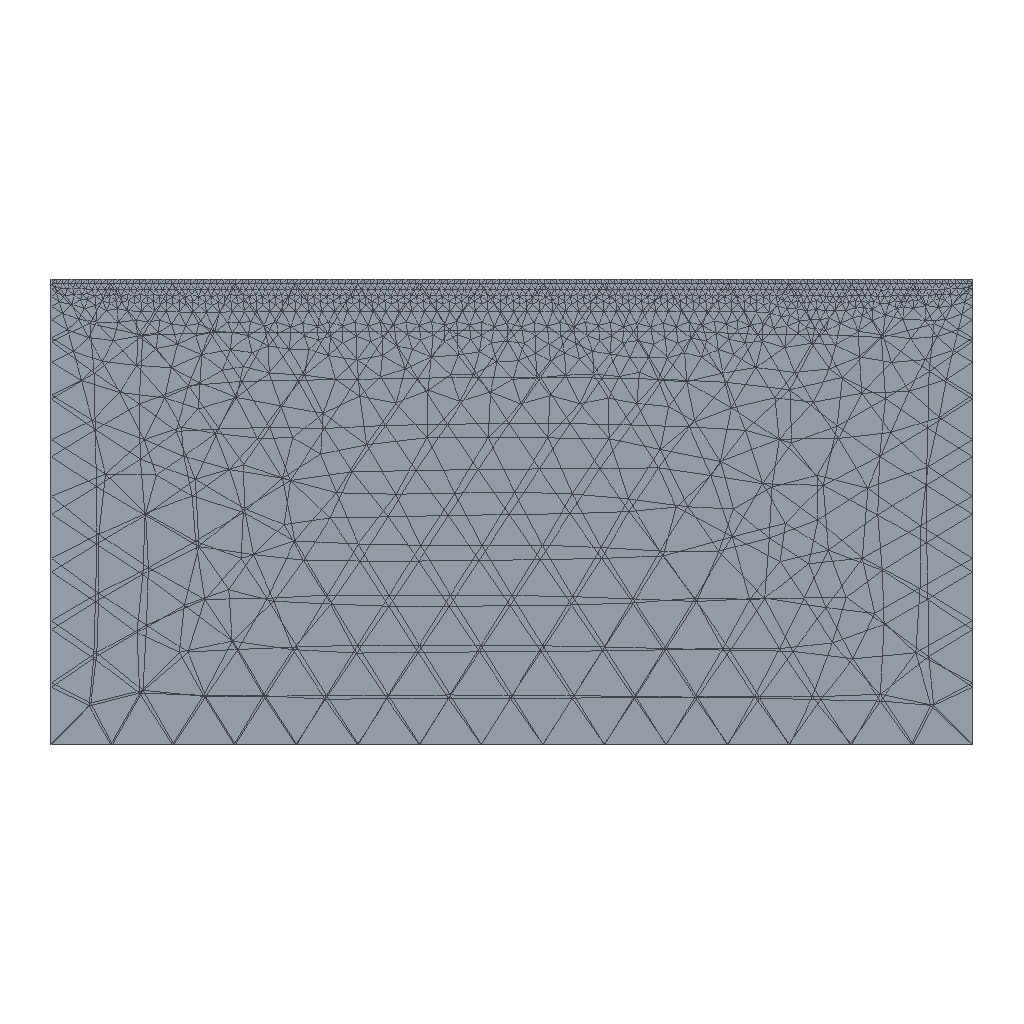Simulation study | comsol
Set-up summary:
category,name,step,type,value,unit,region
solver,comsol,,COMSOL Multiphysics 6.4 (Build: 293)
units,SI; geometry length unit m,,stated,COMSOL default unit system (SI)
analysis,Study 1,,Transient,space_dimension=2D
load_step,std1/time,std1/time,Transient,"type=Transient; times=range(0,5,60)"
analysis,Study 2,,Transient,space_dimension=2D
load_step,std2/time,std2/time,Transient,"type=Transient; times=range(0,5,60)"
mesh,nodes,,,1318
mesh,elements,,,2399
element_type,tri,,,2399
element_type,edg,,,377
element_type,vtx,,,10
component,mod1,,2D,geometry=geom1; domains=1
component,mod2,,2D,geometry=geom2; domains=2
physics,Heat Transfer (ht),mod1,HeatTransfer,"T(T), discontinuousdamagedtissueindicator(discontinuousdamagedtissueindicator), continuousdamagedtissueindicator(continuousdamagedtissueindicator), thermaldamageindicator(thermaldamageindicator), radiativeintensity(radiativeintensity), incidentradiation(incidentradiation), surfaceradiosity(surfaceradiosity)"
physics,Heat Transfer 2 (ht2),mod2,HeatTransfer,"T2(T2), discontinuousdamagedtissueindicator(discontinuousdamagedtissueindicator), continuousdamagedtissueindicator(continuousdamagedtissueindicator), thermaldamageindicator(thermaldamageindicator), radiativeintensity(radiativeintensity), incidentradiation(incidentradiation), surfaceradiosity(surfaceradiosity)"
material,Silica glass,,relpermeability,1,,selection [1]
material,Silica glass,,electricconductivity,1e-14[S/m],,selection [1]
material,Silica glass,,thermalexpansioncoefficient,0.55e-6[1/K],,selection [1]
material,Silica glass,,heatcapacity,703[J/(kg*K)],,selection [1]
material,Silica glass,,relpermittivity,2.09,,selection [1]
material,Silica glass,,density,2203[kg/m^3],,selection [1]
material,Silica glass,,thermalconductivity,1.38[W/(m*K)],,selection [1]
material,Copper,,relpermeability,1,,selection [3]
material,Copper,,electricconductivity,5.998e7[S/m],,selection [3]
material,Copper,,thermalexpansioncoefficient,17e-6[1/K],,selection [3]
material,Copper,,heatcapacity,385[J/(kg*K)],,selection [3]
material,Copper,,relpermittivity,1,,selection [3]
material,Copper,,density,8700[kg/m^3],,selection [3]
material,Copper,,thermalconductivity,400[W/(m*K)],,selection [3]
material,Silica glass (2),,relpermeability,1,,selection [1]
material,Silica glass (2),,electricconductivity,1e-14[S/m],,selection [1]
material,Silica glass (2),,thermalexpansioncoefficient,0.55e-6[1/K],,selection [1]
material,Silica glass (2),,heatcapacity,703[J/(kg*K)],,selection [1]
material,Silica glass (2),,relpermittivity,2.09,,selection [1]
material,Silica glass (2),,density,2203[kg/m^3],,selection [1]
material,Silica glass (2),,thermalconductivity,1.38[W/(m*K)],,selection [1]
material,Copper (2),,relpermeability,1,,selection [2]
material,Copper (2),,electricconductivity,5.998e7[S/m],,selection [2]
material,Copper (2),,thermalexpansioncoefficient,17e-6[1/K],,selection [2]
material,Copper (2),,heatcapacity,385[J/(kg*K)],,selection [2]
material,Copper (2),,relpermittivity,1,,selection [2]
material,Copper (2),,density,8700[kg/m^3],,selection [2]
material,Copper (2),,thermalconductivity,400[W/(m*K)],,selection [2]
bc,Heat Transfer in Solids 1 (solid1),mod1/ht,SolidHeatTransferModel,k=0; rho=0; Cp=0; streamline=0; crosswind=0; pref=1[atm]; hasPhaseChange=0; Solid_material=dommat; u_prime=0 0 0; dfltopaque=1; thermalConductivityModel=Standard,,selection [1]
bc,Thermal Insulation 1 (ins1),mod1/ht,ThermalInsulation,,,selection [2]
bc,Initial Values 1 (init1),mod1/ht,init,Tinit=300[K]; Tinit_resistive=293.15[K],,selection [1]
bc,Continuity (dcont1),mod1/ht,Continuity,pairDisconnect=1; pairSelection=all; pairsList=0,,selection []
bc,Temperature 1 (temp1),mod1/ht,TemperatureBoundary,T0=300[K],,selection [1]
bc,Temperature 2 (temp2),mod1/ht,TemperatureBoundary,T0=600[K],,selection [4]
bc,Highly Conductive Layer 1 (hcl1),mod1/ht,HighlyConductiveLayer,ks=0; rhos=0; Cp_s=0; ds=1e-4; LayerType=Conductive,,selection [3]
bc,Local Thermal Nonequilibrium Boundary 1 (ltneb1),mod1/ht,LocalThermalNonequilibriumBoundary,,,selection []
bc,Heat Transfer in Solids 1 (solid1),mod2/ht2,SolidHeatTransferModel,k=0; rho=0; Cp=0; streamline=0; crosswind=0; pref=1[atm]; hasPhaseChange=0; Solid_material=dommat; u_prime=0 0 0; dfltopaque=1; thermalConductivityModel=Standard,,"selection [1, 2]"
bc,Thermal Insulation 1 (ins1),mod2/ht2,ThermalInsulation,,,"selection [2, 5]"
bc,Initial Values 1 (init1),mod2/ht2,init,Tinit=300[K]; Tinit_resistive=293.15[K],,"selection [1, 2]"
bc,Continuity (dcont1),mod2/ht2,Continuity,pairDisconnect=1; pairSelection=all; pairsList=0,,selection []
bc,Temperature 1 (temp1),mod2/ht2,TemperatureBoundary,T0=300[K],,"selection [1, 3]"
bc,Temperature 2 (temp2),mod2/ht2,TemperatureBoundary,T0=600[K],,"selection [6, 7]"
bc,Local Thermal Nonequilibrium Boundary 1 (ltneb1),mod2/ht2,LocalThermalNonequilibriumBoundary,,,selection []
COMSOL model file for Java, long lists of numbers shortened:
/*
 * em_deck.java
 */

import com.comsol.model.*;
import com.comsol.model.util.*;

/** Model exported on Oct 28 2026, 08:57 by COMSOL 6.4.0.293. */
public class em_deck {

  public static Model run() {
    Model model = ModelUtil.create("Model");

    model.modelPath("");

    model.modelNode().create("mod1");

    model.geom().create("geom1", 2);

    model.mesh().create("mesh1", "geom1");

    model.physics()
         .create("ht", "HeatTransfer", "geom1", new String[]{"I1", "I2", "I3", "I4", "I5", "I6", "I7", "I8", "I9", "I10",
         "I11", "I12"});

    model.study().create("std1");
    model.study("std1").feature().create("time", "Transient");

    model.geom("geom1").feature().create("r1", "Rectangle");
    model.geom("geom1").feature("r1").setIndex("size", "0.02[m]", 0);
    model.geom("geom1").feature("r1").setIndex("size", "0.01[m]", 1);
    model.geom("geom1").runAll();
    model.geom("geom1").run();

    model.material().create("mat1");
    model.material("mat1").name("Silica glass");
    model.material("mat1").propertyGroup("def").set("relpermeability", "1");
    model.material("mat1").propertyGroup("def").set("electricconductivity", "1e-14[S/m]");
    model.material("mat1").propertyGroup("def").set("thermalexpansioncoefficient", "0.55e-6[1/K]");
    model.material("mat1").propertyGroup("def").set("heatcapacity", "703[J/(kg*K)]");
    model.material("mat1").propertyGroup("def").set("relpermittivity", "2.09");
    model.material("mat1").propertyGroup("def").set("density", "2203[kg/m^3]");
    model.material("mat1").propertyGroup("def").set("thermalconductivity", "1.38[W/(m*K)]");
    model.material("mat1").propertyGroup().create("Enu", "Young's modulus and Poisson's ratio");
    model.material("mat1").propertyGroup("Enu").set("poissonsratio", "0.17");
    model.material("mat1").propertyGroup("Enu").set("youngsmodulus", "73.1e9[Pa]");
    model.material("mat1").propertyGroup().create("RefractiveIndex", "Refractive index");
    model.material("mat1").propertyGroup("RefractiveIndex").set("n", "1.45");
    model.material().create("mat2");
    model.material("mat2").name("Copper");
    model.material("mat2").propertyGroup("def").set("relpermeability", "1");
    model.material("mat2").propertyGroup("def").set("electricconductivity", "5.998e7[S/m]");
    model.material("mat2").propertyGroup("def").set("thermalexpansioncoefficient", "17e-6[1/K]");
    model.material("mat2").propertyGroup("def").set("heatcapacity", "385[J/(kg*K)]");
    model.material("mat2").propertyGroup("def").set("relpermittivity", "1");
    model.material("mat2").propertyGroup("def").set("density", "8700[kg/m^3]");
    model.material("mat2").propertyGroup("def").set("thermalconductivity", "400[W/(m*K)]");
    model.material("mat2").propertyGroup().create("Enu", "Young's modulus and Poisson's ratio");
    model.material("mat2").propertyGroup("Enu").set("poissonsratio", "0.35");
    model.material("mat2").propertyGroup("Enu").set("youngsmodulus", "110e9[Pa]");
    model.material("mat2").propertyGroup().create("linzRes", "Linearized resistivity");
    model.material("mat2").propertyGroup("linzRes").set("alpha", "0.0039[1/K]");
    model.material("mat2").propertyGroup("linzRes").set("rho0", "1.72e-8[ohm*m]");
    model.material("mat2").propertyGroup("linzRes").set("Tref", "298[K]");
    model.material("mat2").selection().geom("geom1", 1);
    model.material("mat2").selection().set(new int[]{3});

    model.physics("ht").feature().create("temp1", "TemperatureBoundary", 1);
    model.physics("ht").feature("temp1").selection().set(new int[]{1});
    model.physics("ht").feature("temp1").set("T0", 1, "300[K]");
    model.physics("ht").feature().create("temp2", "TemperatureBoundary", 1);
    model.physics("ht").feature("temp2").selection().set(new int[]{4});
    model.physics("ht").feature("temp2").set("T0", 1, "600[K]");
    model.physics("ht").feature().create("hcl1", "HighlyConductiveLayer", 1);
    model.physics("ht").feature("hcl1").selection().set(new int[]{3});
    model.physics("ht").feature("hcl1").set("ds", 1, "1e-4");
    model.physics("ht").feature("init1").set("T", 1, "300[K]");

    model.mesh("mesh1").feature().create("ftri1", "FreeTri");
    model.mesh("mesh1").run();

    model.study("std1").feature("time").set("tlist", "range(0,5,60)");

    model.sol().create("sol1");
    model.sol("sol1").study("std1");
    model.sol("sol1").feature().create("st1", "StudyStep");
    model.sol("sol1").feature("st1").set("study", "std1");
    model.sol("sol1").feature("st1").set("studystep", "time");
    model.sol("sol1").feature().create("v1", "Variables");
    model.sol("sol1").feature().create("t1", "Time");
    model.sol("sol1").feature("t1").set("tlist", "range(0,5,60)");
    model.sol("sol1").feature("t1").set("plot", "off");
    model.sol("sol1").feature("t1").set("plotfreq", "tout");
    model.sol("sol1").feature("t1").set("probesel", "all");
    model.sol("sol1").feature("t1").set("probes", new String[]{});
    model.sol("sol1").feature("t1").set("probefreq", "tsteps");
    model.sol("sol1").feature("t1").set("estrat", "exclude");
    model.sol("sol1").feature("t1").set("maxorder", 2);
    model.sol("sol1").feature("t1").set("control", "time");
    model.sol("sol1").feature("t1").feature().create("fc1", "FullyCoupled");
    model.sol("sol1").feature("t1").feature("fc1").set("jtech", "once");
    model.sol("sol1").feature("t1").feature("fc1").set("maxiter", 5);
    model.sol("sol1").feature("t1").feature().create("d1", "Direct");
    model.sol("sol1").feature("t1").feature("d1").set("linsolver", "pardiso");
    model.sol("sol1").feature("t1").feature("fc1").set("linsolver", "d1");
    model.sol("sol1").feature("t1").feature("fc1").set("jtech", "once");
    model.sol("sol1").feature("t1").feature("fc1").set("maxiter", 5);
    model.sol("sol1").feature("t1").feature().remove("fcDef");
    model.sol("sol1").attach("std1");

    model.result().create("pg1", 2);
    model.result("pg1").set("data", "dset1");
    model.result("pg1").feature().create("surf1", "Surface");
    model.result("pg1").feature("surf1").set("expr", "T");
    model.result("pg1").feature("surf1").set("descr", "Temperature");

    model.sol("sol1").runAll();

    model.result("pg1").set("windowtitle", "Graphics");
    model.result("pg1").run();

    model.name(".mph");

    model.result("pg1").run();
    model.result("pg1").run();
    model.result("pg1").run();
    model.result("pg1").run();
    model.result("pg1").run();

    model.modelNode().create("mod2");

    model.geom().create("geom2", 2);

    model.mesh().create("mesh2", "geom2");

    model.physics()
         .create("ht2", "HeatTransfer", "geom2", new String[]{"I13", "I14", "I15", "I16", "I17", "I18", "I19", "I20", "I21", "I22",
         "I23", "I24"});

    model.study().create("std2");
    model.study("std2").feature().create("time", "Transient");

    model.geom("geom2").feature().create("r1", "Rectangle");
    model.geom("geom2").feature("r1").setIndex("size", "0.02[m]", 0);
    model.geom("geom2").feature("r1").setIndex("size", "0.01[m]", 1);
    model.geom("geom2").runAll();
    model.geom("geom2").run("r1");
    model.geom("geom2").feature().create("r2", "Rectangle");
    model.geom("geom2").feature("r2").setIndex("size", "0.02[m]", 0);
    model.geom("geom2").feature("r2").setIndex("size", "1e-4[m]", 1);
    model.geom("geom2").feature("r2").setIndex("pos", "0.01[m]", 1);
    model.geom("geom2").runAll();
    model.geom("geom2").run();

    model.material().create("mat3");
    model.material("mat3").name("Silica glass (2)");
    model.material("mat3").propertyGroup("def").set("relpermeability", "1");
    model.material("mat3").propertyGroup("def").set("electricconductivity", "1e-14[S/m]");
    model.material("mat3").propertyGroup("def").set("thermalexpansioncoefficient", "0.55e-6[1/K]");
    model.material("mat3").propertyGroup("def").set("heatcapacity", "703[J/(kg*K)]");
    model.material("mat3").propertyGroup("def").set("relpermittivity", "2.09");
    model.material("mat3").propertyGroup("def").set("density", "2203[kg/m^3]");
    model.material("mat3").propertyGroup("def").set("thermalconductivity", "1.38[W/(m*K)]");
    model.material("mat3").propertyGroup().create("Enu", "Young's modulus and Poisson's ratio");
    model.material("mat3").propertyGroup("Enu").set("poissonsratio", "0.17");
    model.material("mat3").propertyGroup("Enu").set("youngsmodulus", "73.1e9[Pa]");
    model.material("mat3").propertyGroup().create("RefractiveIndex", "Refractive index");
    model.material("mat3").propertyGroup("RefractiveIndex").set("n", "1.45");
    model.material().create("mat4");
    model.material("mat4").name("Copper (2)");
    model.material("mat4").propertyGroup("def").set("relpermeability", "1");
    model.material("mat4").propertyGroup("def").set("electricconductivity", "5.998e7[S/m]");
    model.material("mat4").propertyGroup("def").set("thermalexpansioncoefficient", "17e-6[1/K]");
    model.material("mat4").propertyGroup("def").set("heatcapacity", "385[J/(kg*K)]");
    model.material("mat4").propertyGroup("def").set("relpermittivity", "1");
    model.material("mat4").propertyGroup("def").set("density", "8700[kg/m^3]");
    model.material("mat4").propertyGroup("def").set("thermalconductivity", "400[W/(m*K)]");
    model.material("mat4").propertyGroup().create("Enu", "Young's modulus and Poisson's ratio");
    model.material("mat4").propertyGroup("Enu").set("poissonsratio", "0.35");
    model.material("mat4").propertyGroup("Enu").set("youngsmodulus", "110e9[Pa]");
    model.material("mat4").propertyGroup().create("linzRes", "Linearized resistivity");
    model.material("mat4").propertyGroup("linzRes").set("alpha", "0.0039[1/K]");
    model.material("mat4").propertyGroup("linzRes").set("rho0", "1.72e-8[ohm*m]");
    model.material("mat4").propertyGroup("linzRes").set("Tref", "298[K]");
    model.material("mat3").selection().set(new int[]{1});
    model.material("mat4").selection().set(new int[]{2});

    model.physics("ht2").feature().create("temp1", "TemperatureBoundary", 1);
    model.physics("ht2").feature("temp1").selection().set(new int[]{1, 3});
    model.physics("ht2").feature("temp1").set("T0", 1, "300[K]");
    model.physics("ht2").feature().create("temp2", "TemperatureBoundary", 1);
    model.physics("ht2").feature("temp2").selection().set(new int[]{6, 7});
    model.physics("ht2").feature("temp2").set("T0", 1, "600[K]");
    model.physics("ht2").feature("init1").set("T2", 1, "300[K]");

    model.mesh("mesh2").feature().create("ftri1", "FreeTri");
    model.mesh("mesh2").run();

    model.study("std2").feature("time").set("tlist", "range(0,5,60)");

    model.sol().create("sol2");
    model.sol("sol2").study("std2");
    model.sol("sol2").feature().create("st1", "StudyStep");
    model.sol("sol2").feature("st1").set("study", "std2");
    model.sol("sol2").feature("st1").set("studystep", "time");
    model.sol("sol2").feature().create("v1", "Variables");
    model.sol("sol2").feature().create("t1", "Time");
    model.sol("sol2").feature("t1").set("tlist", "range(0,5,60)");
    model.sol("sol2").feature("t1").set("plot", "off");
    model.sol("sol2").feature("t1").set("plotgroup", "pg1");
    model.sol("sol2").feature("t1").set("plotfreq", "tout");
    model.sol("sol2").feature("t1").set("probesel", "all");
    model.sol("sol2").feature("t1").set("probes", new String[]{});
    model.sol("sol2").feature("t1").set("probefreq", "tsteps");
    model.sol("sol2").feature("t1").set("estrat", "exclude");
    model.sol("sol2").feature("t1").set("maxorder", 2);
    model.sol("sol2").feature("t1").set("control", "time");
    model.sol("sol2").feature("t1").feature().create("seDef", "Segregated");
    model.sol("sol2").feature("t1").feature().create("fc1", "FullyCoupled");
    model.sol("sol2").feature("t1").feature("fc1").set("jtech", "once");
    model.sol("sol2").feature("t1").feature("fc1").set("maxiter", 5);
    model.sol("sol2").feature("t1").feature().create("d1", "Direct");
    model.sol("sol2").feature("t1").feature("d1").set("linsolver", "pardiso");
    model.sol("sol2").feature("t1").feature("fc1").set("linsolver", "d1");
    model.sol("sol2").feature("t1").feature("fc1").set("jtech", "once");
    model.sol("sol2").feature("t1").feature("fc1").set("maxiter", 5);
    model.sol("sol2").feature("t1").feature().remove("fcDef");
    model.sol("sol2").feature("t1").feature().remove("seDef");
    model.sol("sol2").attach("std2");

    model.result().create("pg2", 2);
    model.result("pg2").set("data", "dset2");
    model.result("pg2").feature().create("surf1", "Surface");
    model.result("pg2").feature("surf1").set("expr", "T");
    model.result("pg2").feature("surf1").set("descr", "Temperature");

    model.sol("sol2").runAll();

    model.result("pg2").run();

    model.name(".mph");

    model.result("pg2").run();
    model.result("pg2").set("windowtitleactive", "on");
    model.result("pg2").set("windowtitle", "Copper Layer Plot");
    model.result("pg2").set("window", "new");
    model.result("pg1").set("windowtitle", "Graphics");
    model.result("pg2").set("window", "window1");
    model.result("pg2").run();

    model.label("in.mph");

    return model;
  }

  public static void main(String[] args) {
    run();
  }

}
Results summary:
result,max T = abs(mod1.T),dset1 (13 solution(s)),,600,K
result,max T = abs(mod1.T),dset2 (13 solution(s)),,600,K
result,max T2 = abs(mod2.T2),dset3 (13 solution(s)),,600,K